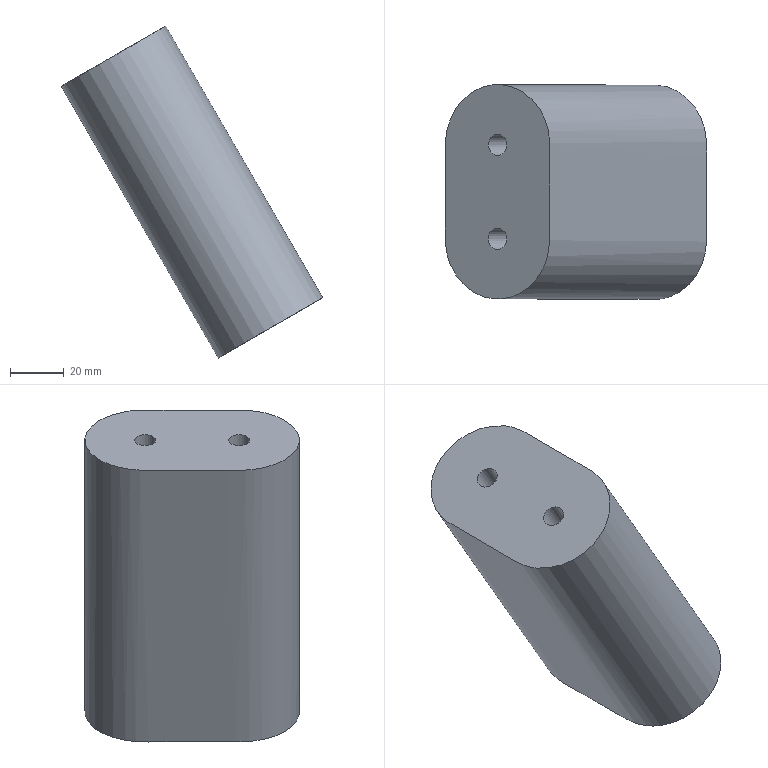Part | NX | features solid 2 | 1 solid | 7 faces | box 97.511 x 79.969 x 123.814 mm | volume 367586 mm3 | plane 2 | cone 2 | cylinder 2 | spline 1 | commonest cylinder face diameters 8 x2